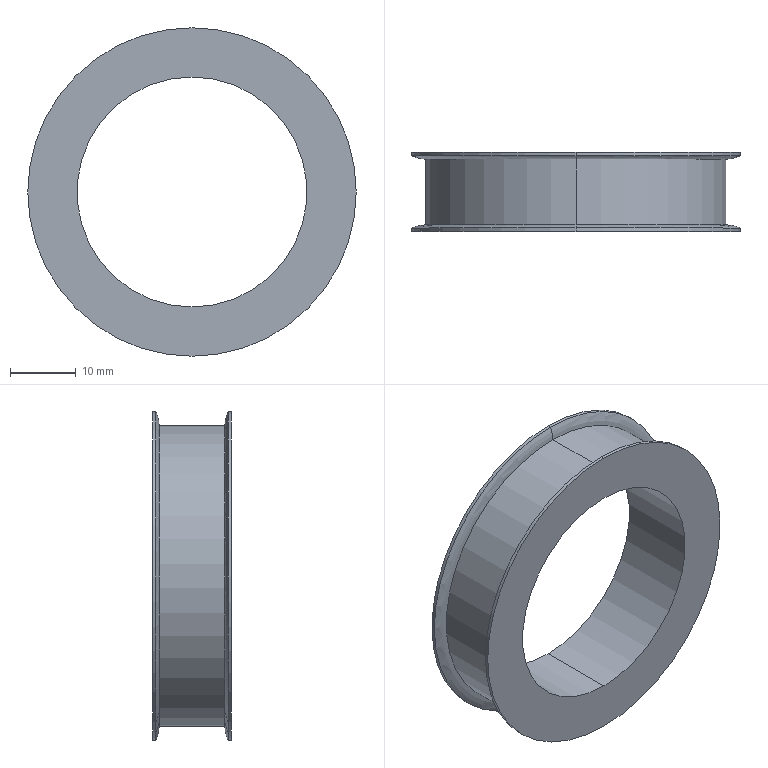Part | SolidWorks | features Revolution 2 | 1 solid | 14 faces | box 50 x 12 x 50 mm | volume 8776 mm3 | cylinder 8 | torus 4 | plane 2 | commonest cylinder face diameters 50 x4 35 x2 45.84 x2
STEP:
#1=CARTESIAN_POINT('',(0.,-5.5,-25.));
#2=VERTEX_POINT('',#1);
#3=CARTESIAN_POINT('',(0.,-5.5,25.));
#4=VERTEX_POINT('',#3);
#5=CARTESIAN_POINT('',(0.,-5.5,0.));
#6=DIRECTION('',(0.,-1.,0.));
#7=DIRECTION('',(0.,0.,-1.));
#8=AXIS2_PLACEMENT_3D('',#5,#6,#7);
#9=CIRCLE('',#8,25.);
#10=EDGE_CURVE('',#2,#4,#9,.T.);
#11=ORIENTED_EDGE('',*,*,#10,.T.);
#12=CARTESIAN_POINT('',(0.,-6.,25.));
#13=VERTEX_POINT('',#12);
#14=CARTESIAN_POINT('',(0.,0.,25.));
#15=DIRECTION('',(0.,-1.,0.));
#16=VECTOR('',#15,1000.);
#17=LINE('',#14,#16);
#18=EDGE_CURVE('',#4,#13,#17,.T.);
#19=ORIENTED_EDGE('',*,*,#18,.T.);
#20=CARTESIAN_POINT('',(0.,-6.,-25.));
#21=VERTEX_POINT('',#20);
#22=CARTESIAN_POINT('',(0.,-6.,0.));
#23=DIRECTION('',(0.,-1.,0.));
#24=DIRECTION('',(0.,0.,-1.));
#25=AXIS2_PLACEMENT_3D('',#22,#23,#24);
#26=CIRCLE('',#25,25.);
#27=EDGE_CURVE('',#21,#13,#26,.T.);
#28=ORIENTED_EDGE('',*,*,#27,.F.);
#29=CARTESIAN_POINT('',(0.,0.,-25.));
#30=DIRECTION('',(0.,-1.,0.));
#31=VECTOR('',#30,1000.);
#32=LINE('',#29,#31);
#33=EDGE_CURVE('',#2,#21,#32,.T.);
#34=ORIENTED_EDGE('',*,*,#33,.F.);
#35=EDGE_LOOP('',(#11,#19,#28,#34));
#36=FACE_OUTER_BOUND('',#35,.T.);
#37=CARTESIAN_POINT('',(0.,0.,0.));
#38=DIRECTION('',(0.,-1.,0.));
#39=DIRECTION('',(0.,0.,-1.));
#40=AXIS2_PLACEMENT_3D('',#37,#38,#39);
#41=CYLINDRICAL_SURFACE('',#40,25.);
#42=ADVANCED_FACE('',(#36),#41,.T.);
#43=CARTESIAN_POINT('',(0.,-5.,-22.92));
#44=VERTEX_POINT('',#43);
#45=CARTESIAN_POINT('',(0.,-5.,22.92));
#46=VERTEX_POINT('',#45);
#47=CARTESIAN_POINT('',(0.,-5.,0.));
#48=DIRECTION('',(0.,-1.,0.));
#49=DIRECTION('',(0.,0.,-1.));
#50=AXIS2_PLACEMENT_3D('',#47,#48,#49);
#51=CIRCLE('',#50,22.92);
#52=EDGE_CURVE('',#44,#46,#51,.T.);
#53=ORIENTED_EDGE('',*,*,#52,.T.);
#54=CARTESIAN_POINT('',(0.,-9.999,22.818));
#55=DIRECTION('',(1.,0.,0.));
#56=DIRECTION('',(0.,0.,-1.));
#57=AXIS2_PLACEMENT_3D('',#54,#55,#56);
#58=CIRCLE('',#57,5.);
#59=EDGE_CURVE('',#46,#4,#58,.T.);
#60=ORIENTED_EDGE('',*,*,#59,.T.);
#61=ORIENTED_EDGE('',*,*,#10,.F.);
#62=CARTESIAN_POINT('',(0.,-9.999,-22.818));
#63=DIRECTION('',(-1.,0.,0.));
#64=DIRECTION('',(0.,0.,1.));
#65=AXIS2_PLACEMENT_3D('',#62,#63,#64);
#66=CIRCLE('',#65,5.);
#67=EDGE_CURVE('',#44,#2,#66,.T.);
#68=ORIENTED_EDGE('',*,*,#67,.F.);
#69=EDGE_LOOP('',(#53,#60,#61,#68));
#70=FACE_OUTER_BOUND('',#69,.T.);
#71=CARTESIAN_POINT('',(0.,-9.999,0.));
#72=DIRECTION('',(0.,-1.,0.));
#73=DIRECTION('',(0.,0.,-1.));
#74=AXIS2_PLACEMENT_3D('',#71,#72,#73);
#75=TOROIDAL_SURFACE('',#74,22.818,5.);
#76=ADVANCED_FACE('',(#70),#75,.T.);
#77=CARTESIAN_POINT('',(0.,6.,-25.));
#78=VERTEX_POINT('',#77);
#79=CARTESIAN_POINT('',(0.,6.,25.));
#80=VERTEX_POINT('',#79);
#81=CARTESIAN_POINT('',(0.,6.,0.));
#82=DIRECTION('',(0.,-1.,0.));
#83=DIRECTION('',(0.,0.,-1.));
#84=AXIS2_PLACEMENT_3D('',#81,#82,#83);
#85=CIRCLE('',#84,25.);
#86=EDGE_CURVE('',#78,#80,#85,.T.);
#87=ORIENTED_EDGE('',*,*,#86,.T.);
#88=CARTESIAN_POINT('',(0.,5.5,25.));
#89=VERTEX_POINT('',#88);
#90=CARTESIAN_POINT('',(0.,0.,25.));
#91=DIRECTION('',(0.,-1.,0.));
#92=VECTOR('',#91,1000.);
#93=LINE('',#90,#92);
#94=EDGE_CURVE('',#80,#89,#93,.T.);
#95=ORIENTED_EDGE('',*,*,#94,.T.);
#96=CARTESIAN_POINT('',(0.,5.5,-25.));
#97=VERTEX_POINT('',#96);
#98=CARTESIAN_POINT('',(0.,5.5,0.));
#99=DIRECTION('',(0.,-1.,0.));
#100=DIRECTION('',(0.,0.,-1.));
#101=AXIS2_PLACEMENT_3D('',#98,#99,#100);
#102=CIRCLE('',#101,25.);
#103=EDGE_CURVE('',#97,#89,#102,.T.);
#104=ORIENTED_EDGE('',*,*,#103,.F.);
#105=CARTESIAN_POINT('',(0.,0.,-25.));
#106=DIRECTION('',(0.,-1.,0.));
#107=VECTOR('',#106,1000.);
#108=LINE('',#105,#107);
#109=EDGE_CURVE('',#78,#97,#108,.T.);
#110=ORIENTED_EDGE('',*,*,#109,.F.);
#111=EDGE_LOOP('',(#87,#95,#104,#110));
#112=FACE_OUTER_BOUND('',#111,.T.);
#113=CARTESIAN_POINT('',(0.,0.,0.));
#114=DIRECTION('',(0.,-1.,0.));
#115=DIRECTION('',(0.,0.,-1.));
#116=AXIS2_PLACEMENT_3D('',#113,#114,#115);
#117=CYLINDRICAL_SURFACE('',#116,25.);
#118=ADVANCED_FACE('',(#112),#117,.T.);
#119=ORIENTED_EDGE('',*,*,#103,.T.);
#120=CARTESIAN_POINT('',(0.,5.,22.92));
#121=VERTEX_POINT('',#120);
#122=CARTESIAN_POINT('',(0.,9.999,22.818));
#123=DIRECTION('',(1.,0.,0.));
#124=DIRECTION('',(0.,0.,-1.));
#125=AXIS2_PLACEMENT_3D('',#122,#123,#124);
#126=CIRCLE('',#125,5.);
#127=EDGE_CURVE('',#89,#121,#126,.T.);
#128=ORIENTED_EDGE('',*,*,#127,.T.);
#129=CARTESIAN_POINT('',(0.,5.,-22.92));
#130=VERTEX_POINT('',#129);
#131=CARTESIAN_POINT('',(0.,5.,0.));
#132=DIRECTION('',(0.,-1.,0.));
#133=DIRECTION('',(0.,0.,-1.));
#134=AXIS2_PLACEMENT_3D('',#131,#132,#133);
#135=CIRCLE('',#134,22.92);
#136=EDGE_CURVE('',#130,#121,#135,.T.);
#137=ORIENTED_EDGE('',*,*,#136,.F.);
#138=CARTESIAN_POINT('',(0.,9.999,-22.818));
#139=DIRECTION('',(-1.,0.,0.));
#140=DIRECTION('',(0.,0.,1.));
#141=AXIS2_PLACEMENT_3D('',#138,#139,#140);
#142=CIRCLE('',#141,5.);
#143=EDGE_CURVE('',#97,#130,#142,.T.);
#144=ORIENTED_EDGE('',*,*,#143,.F.);
#145=EDGE_LOOP('',(#119,#128,#137,#144));
#146=FACE_OUTER_BOUND('',#145,.T.);
#147=CARTESIAN_POINT('',(0.,9.999,0.));
#148=DIRECTION('',(0.,-1.,0.));
#149=DIRECTION('',(0.,0.,-1.));
#150=AXIS2_PLACEMENT_3D('',#147,#148,#149);
#151=TOROIDAL_SURFACE('',#150,22.818,5.);
#152=ADVANCED_FACE('',(#146),#151,.T.);
#153=ORIENTED_EDGE('',*,*,#136,.T.);
#154=CARTESIAN_POINT('',(0.,0.,22.92));
#155=DIRECTION('',(0.,-1.,0.));
#156=VECTOR('',#155,1000.);
#157=LINE('',#154,#156);
#158=EDGE_CURVE('',#121,#46,#157,.T.);
#159=ORIENTED_EDGE('',*,*,#158,.T.);
#160=ORIENTED_EDGE('',*,*,#52,.F.);
#161=CARTESIAN_POINT('',(0.,0.,-22.92));
#162=DIRECTION('',(0.,-1.,0.));
#163=VECTOR('',#162,1000.);
#164=LINE('',#161,#163);
#165=EDGE_CURVE('',#130,#44,#164,.T.);
#166=ORIENTED_EDGE('',*,*,#165,.F.);
#167=EDGE_LOOP('',(#153,#159,#160,#166));
#168=FACE_OUTER_BOUND('',#167,.T.);
#169=CARTESIAN_POINT('',(0.,0.,0.));
#170=DIRECTION('',(0.,-1.,0.));
#171=DIRECTION('',(0.,0.,-1.));
#172=AXIS2_PLACEMENT_3D('',#169,#170,#171);
#173=CYLINDRICAL_SURFACE('',#172,22.92);
#174=ADVANCED_FACE('',(#168),#173,.T.);
#175=CARTESIAN_POINT('',(0.,6.,17.5));
#176=VERTEX_POINT('',#175);
#177=CARTESIAN_POINT('',(0.,6.,-17.5));
#178=VERTEX_POINT('',#177);
#179=CARTESIAN_POINT('',(0.,6.,0.));
#180=DIRECTION('',(0.,-1.,0.));
#181=DIRECTION('',(0.,0.,-1.));
#182=AXIS2_PLACEMENT_3D('',#179,#180,#181);
#183=CIRCLE('',#182,17.5);
#184=EDGE_CURVE('',#176,#178,#183,.T.);
#185=ORIENTED_EDGE('',*,*,#184,.F.);
#186=CARTESIAN_POINT('',(0.,-6.,17.5));
#187=VERTEX_POINT('',#186);
#188=CARTESIAN_POINT('',(0.,0.,17.5));
#189=DIRECTION('',(0.,-1.,0.));
#190=VECTOR('',#189,1000.);
#191=LINE('',#188,#190);
#192=EDGE_CURVE('',#176,#187,#191,.T.);
#193=ORIENTED_EDGE('',*,*,#192,.T.);
#194=CARTESIAN_POINT('',(0.,-6.,-17.5));
#195=VERTEX_POINT('',#194);
#196=CARTESIAN_POINT('',(0.,-6.,0.));
#197=DIRECTION('',(0.,-1.,0.));
#198=DIRECTION('',(0.,0.,-1.));
#199=AXIS2_PLACEMENT_3D('',#196,#197,#198);
#200=CIRCLE('',#199,17.5);
#201=EDGE_CURVE('',#187,#195,#200,.T.);
#202=ORIENTED_EDGE('',*,*,#201,.T.);
#203=CARTESIAN_POINT('',(0.,0.,-17.5));
#204=DIRECTION('',(0.,-1.,0.));
#205=VECTOR('',#204,1000.);
#206=LINE('',#203,#205);
#207=EDGE_CURVE('',#178,#195,#206,.T.);
#208=ORIENTED_EDGE('',*,*,#207,.F.);
#209=EDGE_LOOP('',(#185,#193,#202,#208));
#210=FACE_OUTER_BOUND('',#209,.T.);
#211=CARTESIAN_POINT('',(0.,0.,0.));
#212=DIRECTION('',(0.,-1.,0.));
#213=DIRECTION('',(0.,0.,-1.));
#214=AXIS2_PLACEMENT_3D('',#211,#212,#213);
#215=CYLINDRICAL_SURFACE('',#214,17.5);
#216=ADVANCED_FACE('',(#210),#215,.F.);
#217=CARTESIAN_POINT('',(0.,6.,0.));
#218=DIRECTION('',(0.,-1.,0.));
#219=DIRECTION('',(0.,0.,-1.));
#220=AXIS2_PLACEMENT_3D('',#217,#218,#219);
#221=CIRCLE('',#220,17.5);
#222=EDGE_CURVE('',#178,#176,#221,.T.);
#223=ORIENTED_EDGE('',*,*,#222,.T.);
#224=ORIENTED_EDGE('',*,*,#184,.T.);
#225=EDGE_LOOP('',(#223,#224));
#226=FACE_BOUND('',#225,.T.);
#227=ORIENTED_EDGE('',*,*,#86,.F.);
#228=CARTESIAN_POINT('',(0.,6.,0.));
#229=DIRECTION('',(0.,-1.,0.));
#230=DIRECTION('',(0.,0.,-1.));
#231=AXIS2_PLACEMENT_3D('',#228,#229,#230);
#232=CIRCLE('',#231,25.);
#233=EDGE_CURVE('',#80,#78,#232,.T.);
#234=ORIENTED_EDGE('',*,*,#233,.F.);
#235=EDGE_LOOP('',(#227,#234));
#236=FACE_OUTER_BOUND('',#235,.T.);
#237=CARTESIAN_POINT('',(20.,6.,0.));
#238=DIRECTION('',(0.,1.,0.));
#239=DIRECTION('',(0.,0.,1.));
#240=AXIS2_PLACEMENT_3D('',#237,#238,#239);
#241=PLANE('',#240);
#242=ADVANCED_FACE('',(#226,#236),#241,.T.);
#243=ORIENTED_EDGE('',*,*,#192,.F.);
#244=ORIENTED_EDGE('',*,*,#222,.F.);
#245=ORIENTED_EDGE('',*,*,#207,.T.);
#246=CARTESIAN_POINT('',(0.,-6.,0.));
#247=DIRECTION('',(0.,-1.,0.));
#248=DIRECTION('',(0.,0.,-1.));
#249=AXIS2_PLACEMENT_3D('',#246,#247,#248);
#250=CIRCLE('',#249,17.5);
#251=EDGE_CURVE('',#195,#187,#250,.T.);
#252=ORIENTED_EDGE('',*,*,#251,.T.);
#253=EDGE_LOOP('',(#243,#244,#245,#252));
#254=FACE_OUTER_BOUND('',#253,.T.);
#255=CARTESIAN_POINT('',(0.,0.,0.));
#256=DIRECTION('',(0.,-1.,0.));
#257=DIRECTION('',(0.,0.,-1.));
#258=AXIS2_PLACEMENT_3D('',#255,#256,#257);
#259=CYLINDRICAL_SURFACE('',#258,17.5);
#260=ADVANCED_FACE('',(#254),#259,.F.);
#261=ORIENTED_EDGE('',*,*,#251,.F.);
#262=ORIENTED_EDGE('',*,*,#201,.F.);
#263=EDGE_LOOP('',(#261,#262));
#264=FACE_BOUND('',#263,.T.);
#265=ORIENTED_EDGE('',*,*,#27,.T.);
#266=CARTESIAN_POINT('',(0.,-6.,0.));
#267=DIRECTION('',(0.,-1.,0.));
#268=DIRECTION('',(0.,0.,-1.));
#269=AXIS2_PLACEMENT_3D('',#266,#267,#268);
#270=CIRCLE('',#269,25.);
#271=EDGE_CURVE('',#13,#21,#270,.T.);
#272=ORIENTED_EDGE('',*,*,#271,.T.);
#273=EDGE_LOOP('',(#265,#272));
#274=FACE_OUTER_BOUND('',#273,.T.);
#275=CARTESIAN_POINT('',(20.,-6.,0.));
#276=DIRECTION('',(0.,1.,0.));
#277=DIRECTION('',(0.,0.,1.));
#278=AXIS2_PLACEMENT_3D('',#275,#276,#277);
#279=PLANE('',#278);
#280=ADVANCED_FACE('',(#264,#274),#279,.F.);
#281=ORIENTED_EDGE('',*,*,#158,.F.);
#282=CARTESIAN_POINT('',(0.,5.,0.));
#283=DIRECTION('',(0.,-1.,0.));
#284=DIRECTION('',(0.,0.,-1.));
#285=AXIS2_PLACEMENT_3D('',#282,#283,#284);
#286=CIRCLE('',#285,22.92);
#287=EDGE_CURVE('',#121,#130,#286,.T.);
#288=ORIENTED_EDGE('',*,*,#287,.T.);
#289=ORIENTED_EDGE('',*,*,#165,.T.);
#290=CARTESIAN_POINT('',(0.,-5.,0.));
#291=DIRECTION('',(0.,-1.,0.));
#292=DIRECTION('',(0.,0.,-1.));
#293=AXIS2_PLACEMENT_3D('',#290,#291,#292);
#294=CIRCLE('',#293,22.92);
#295=EDGE_CURVE('',#46,#44,#294,.T.);
#296=ORIENTED_EDGE('',*,*,#295,.F.);
#297=EDGE_LOOP('',(#281,#288,#289,#296));
#298=FACE_OUTER_BOUND('',#297,.T.);
#299=CARTESIAN_POINT('',(0.,0.,0.));
#300=DIRECTION('',(0.,-1.,0.));
#301=DIRECTION('',(0.,0.,-1.));
#302=AXIS2_PLACEMENT_3D('',#299,#300,#301);
#303=CYLINDRICAL_SURFACE('',#302,22.92);
#304=ADVANCED_FACE('',(#298),#303,.T.);
#305=ORIENTED_EDGE('',*,*,#127,.F.);
#306=CARTESIAN_POINT('',(0.,5.5,0.));
#307=DIRECTION('',(0.,-1.,0.));
#308=DIRECTION('',(0.,0.,-1.));
#309=AXIS2_PLACEMENT_3D('',#306,#307,#308);
#310=CIRCLE('',#309,25.);
#311=EDGE_CURVE('',#89,#97,#310,.T.);
#312=ORIENTED_EDGE('',*,*,#311,.T.);
#313=ORIENTED_EDGE('',*,*,#143,.T.);
#314=ORIENTED_EDGE('',*,*,#287,.F.);
#315=EDGE_LOOP('',(#305,#312,#313,#314));
#316=FACE_OUTER_BOUND('',#315,.T.);
#317=CARTESIAN_POINT('',(0.,9.999,0.));
#318=DIRECTION('',(0.,-1.,0.));
#319=DIRECTION('',(0.,0.,-1.));
#320=AXIS2_PLACEMENT_3D('',#317,#318,#319);
#321=TOROIDAL_SURFACE('',#320,22.818,5.);
#322=ADVANCED_FACE('',(#316),#321,.T.);
#323=ORIENTED_EDGE('',*,*,#94,.F.);
#324=ORIENTED_EDGE('',*,*,#233,.T.);
#325=ORIENTED_EDGE('',*,*,#109,.T.);
#326=ORIENTED_EDGE('',*,*,#311,.F.);
#327=EDGE_LOOP('',(#323,#324,#325,#326));
#328=FACE_OUTER_BOUND('',#327,.T.);
#329=CARTESIAN_POINT('',(0.,0.,0.));
#330=DIRECTION('',(0.,-1.,0.));
#331=DIRECTION('',(0.,0.,-1.));
#332=AXIS2_PLACEMENT_3D('',#329,#330,#331);
#333=CYLINDRICAL_SURFACE('',#332,25.);
#334=ADVANCED_FACE('',(#328),#333,.T.);
#335=ORIENTED_EDGE('',*,*,#59,.F.);
#336=ORIENTED_EDGE('',*,*,#295,.T.);
#337=ORIENTED_EDGE('',*,*,#67,.T.);
#338=CARTESIAN_POINT('',(0.,-5.5,0.));
#339=DIRECTION('',(0.,-1.,0.));
#340=DIRECTION('',(0.,0.,-1.));
#341=AXIS2_PLACEMENT_3D('',#338,#339,#340);
#342=CIRCLE('',#341,25.);
#343=EDGE_CURVE('',#4,#2,#342,.T.);
#344=ORIENTED_EDGE('',*,*,#343,.F.);
#345=EDGE_LOOP('',(#335,#336,#337,#344));
#346=FACE_OUTER_BOUND('',#345,.T.);
#347=CARTESIAN_POINT('',(0.,-9.999,0.));
#348=DIRECTION('',(0.,-1.,0.));
#349=DIRECTION('',(0.,0.,-1.));
#350=AXIS2_PLACEMENT_3D('',#347,#348,#349);
#351=TOROIDAL_SURFACE('',#350,22.818,5.);
#352=ADVANCED_FACE('',(#346),#351,.T.);
#353=ORIENTED_EDGE('',*,*,#18,.F.);
#354=ORIENTED_EDGE('',*,*,#343,.T.);
#355=ORIENTED_EDGE('',*,*,#33,.T.);
#356=ORIENTED_EDGE('',*,*,#271,.F.);
#357=EDGE_LOOP('',(#353,#354,#355,#356));
#358=FACE_OUTER_BOUND('',#357,.T.);
#359=CARTESIAN_POINT('',(0.,0.,0.));
#360=DIRECTION('',(0.,-1.,0.));
#361=DIRECTION('',(0.,0.,-1.));
#362=AXIS2_PLACEMENT_3D('',#359,#360,#361);
#363=CYLINDRICAL_SURFACE('',#362,25.);
#364=ADVANCED_FACE('',(#358),#363,.T.);
#365=CLOSED_SHELL('',(#42,#76,#118,#152,#174,#216,#242,#260,#280,#304,#322,#334,#352,#364));
#366=MANIFOLD_SOLID_BREP('',#365);
#367=CARTESIAN_POINT('',(0.,0.,0.));
#368=DIRECTION('',(0.,0.,1.));
#369=DIRECTION('',(1.,0.,0.));
#370=AXIS2_PLACEMENT_3D('',#367,#368,#369);
#371=(LENGTH_UNIT()NAMED_UNIT(*)SI_UNIT(.MILLI.,.METRE.));
#372=UNCERTAINTY_MEASURE_WITH_UNIT(LENGTH_MEASURE(0.00001),#371,'','');
#373=(NAMED_UNIT(*)PLANE_ANGLE_UNIT()SI_UNIT($,.RADIAN.));
#374=(NAMED_UNIT(*)SI_UNIT($,.STERADIAN.)SOLID_ANGLE_UNIT());
#375=(GEOMETRIC_REPRESENTATION_CONTEXT(3)GLOBAL_UNCERTAINTY_ASSIGNED_CONTEXT((#372))GLOBAL_UNIT_ASSIGNED_CONTEXT((#371,#373,#374))REPRESENTATION_CONTEXT('',''));
#376=ADVANCED_BREP_SHAPE_REPRESENTATION('',(#366,#370),#375);